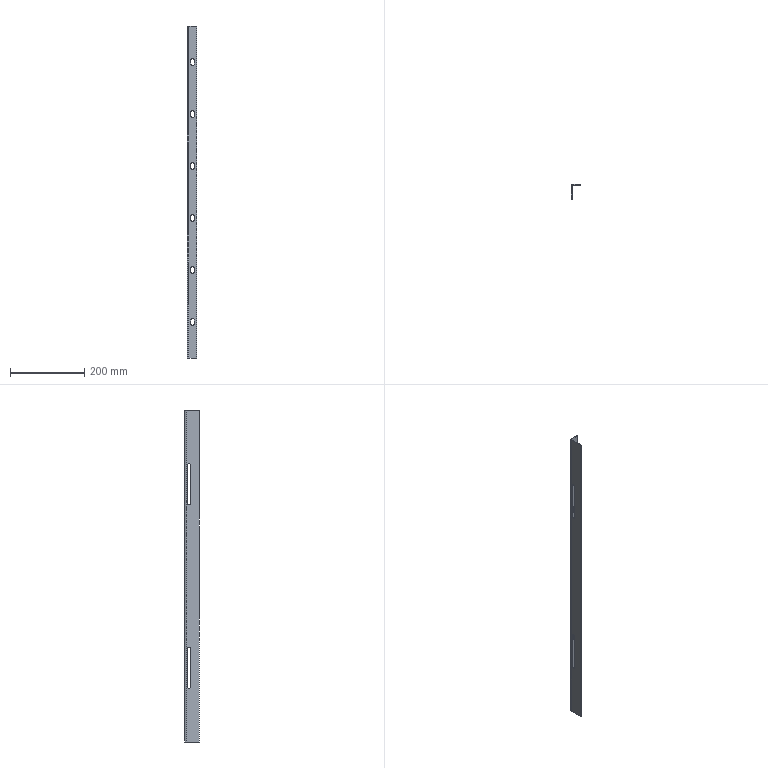Part | SolidWorks | features ICE 2, FlatPattern 1, SMBaseFlange 1, SheetMetal 1 | 1 solid | 54 faces | box 25 x 40 x 895 mm | volume 104308 mm3 | plane 28 | cylinder 26 | commonest cylinder face diameters 9 x18 10 x6 4 x1 8 x1